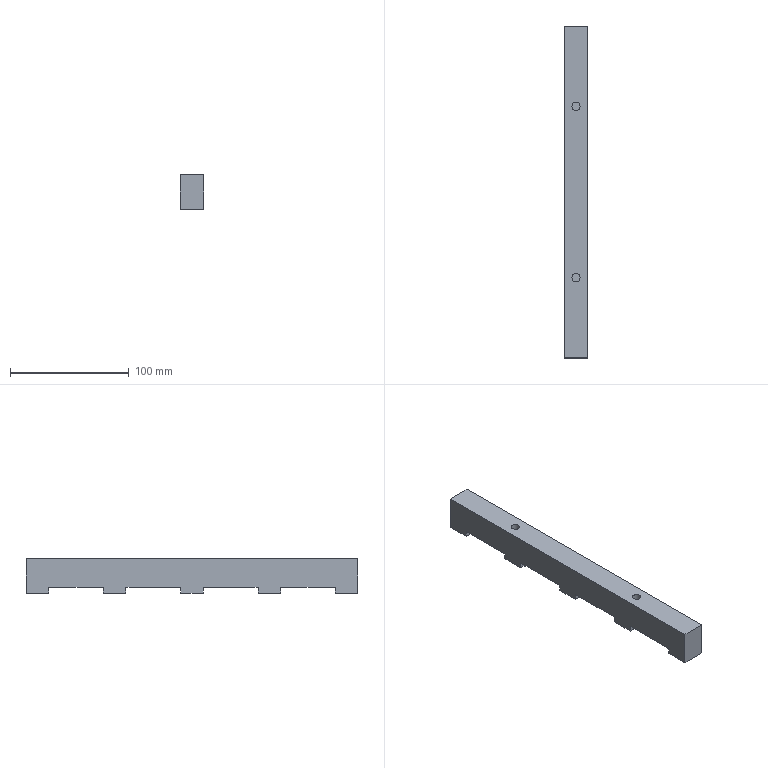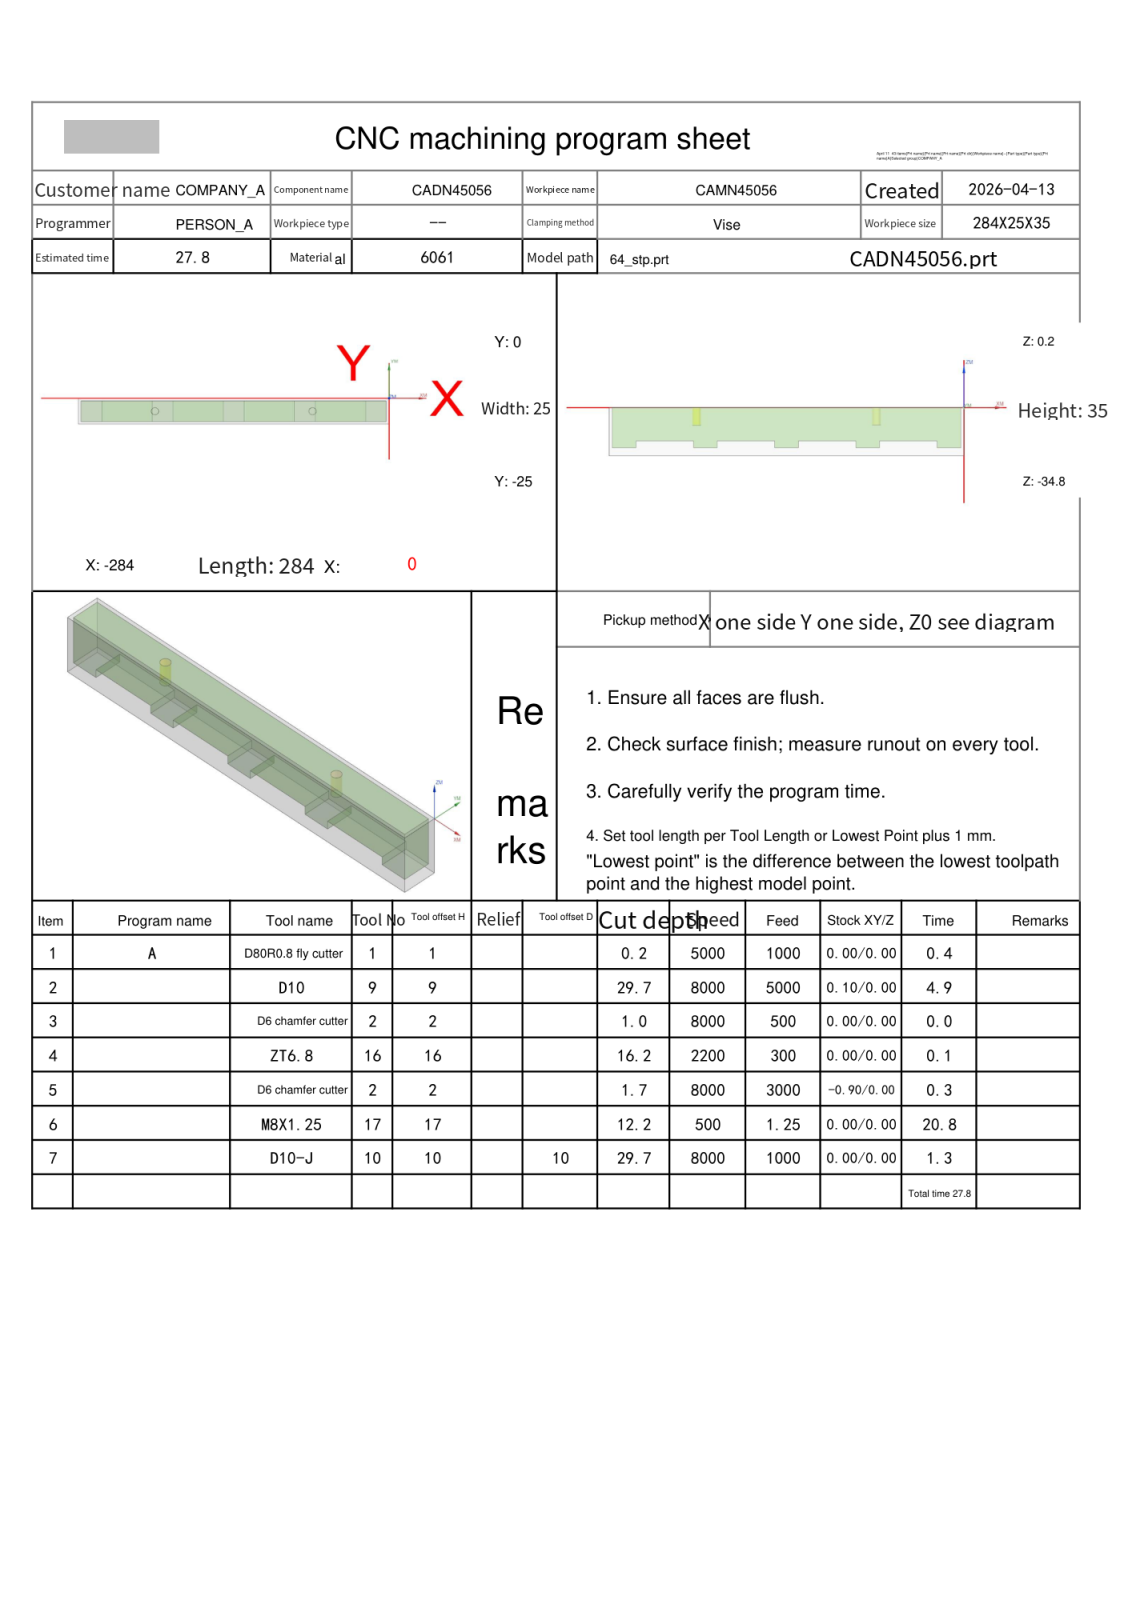NC program | NX | posted by the shop | part box 20 x 279 x 29 mm
Whole program:
%
O0001
(Machine time: 48.52 MIN)
(===Total Tool:6===)
(T1=D80R0.8 fly cutter D=80.  R=0.8  D-  H01 Z=-0.   )
(T9=D10     D=10.  R=0.   D-  H09 Z=-29.5 )
(T2=D6 chamfer cutter   D=6.   R=0.   D-  H02 Z=-1.5  )
(T16=ZT6.8  D=6.8  DR_a=118 D-  H16 Z=-16.  )
(T17=M8X1.25 D=6.8  DR_a=180 D-  H17 Z=-12.  )
(T10=D10-J  D=10.  R=0.   D10 H10 Z=-29.5 )
G80 G90 G17 G49 G40
G91 G28 Z0
M01
N1 T01 M06
(D80R0.8 fly cutter  D=80. R=0.8 H=01 ce=0.00 di=0.00)
G00 G90 G54 X-326.5 Y-12.5 M03 S5000
G43 H01 Z20.
M08
Z2.
G01 Z0.0 F1000.
X-321.5
X37.5
X42.5
Z2.
G00 Z20.
G91 G28 Z0.0
M05
M09
G91 G28 Z0.0
M01
N2 T09 M06
(D10  D=10. R=0. H=09 ce=0.10 di=0.00)
G00 G90 G54 X-142. Y2.6 M03 S8000
G43 H09 Z20.
M08
Z.5
G01 X-2.5 Z.325 F5000.
G02 X2.6 Y-2.5 Z.315 I0.0 J-5.1
G01 Y-22.5 Z.29
G02 X-2.5 Y-27.6 Z.28 I-5.1 J0.0
G01 X-281.5 Z-.07
G02 X-286.6 Y-22.5 Z-.08 I0.0 J5.1
G01 Y-2.5 Z-.105
G02 X-281.5 Y2.6 Z-.115 I5.1 J0.0
G01 X-2.5 Z-.464
G02 X2.6 Y-2.5 Z-.474 I0.0 J-5.1
G01 Y-22.5 Z-.499
G02 X-2.5 Y-27.6 Z-.509 I-5.1 J0.0
G01 X-281.5 Z-.859
G02 X-286.6 Y-22.5 Z-.869 I0.0 J5.1
G01 Y-2.5 Z-.894
G02 X-281.5 Y2.6 Z-.904 I5.1 J0.0
G01 X-2.5 Z-1.254
G02 X2.6 Y-2.5 Z-1.264 I0.0 J-5.1
G01 Y-22.5 Z-1.289
G02 X-2.5 Y-27.6 Z-1.299 I-5.1 J0.0
G01 X-281.5 Z-1.648
G02 X-286.6 Y-22.5 Z-1.659 I0.0 J5.1
G01 Y-2.5 Z-1.684
G02 X-281.5 Y2.6 Z-1.694 I5.1 J0.0
G01 X-2.5 Z-2.043
G02 X2.6 Y-2.5 Z-2.053 I0.0 J-5.1
G01 Y-22.5 Z-2.078
G02 X-2.5 Y-27.6 Z-2.088 I-5.1 J0.0
G01 X-281.5 Z-2.438
G02 X-286.6 Y-22.5 Z-2.448 I0.0 J5.1
G01 Y-2.5 Z-2.473
G02 X-281.5 Y2.6 Z-2.483 I5.1 J0.0
G01 X-2.5 Z-2.833
G02 X2.6 Y-2.5 Z-2.843 I0.0 J-5.1
G01 Y-22.5 Z-2.868
G02 X-2.5 Y-27.6 Z-2.878 I-5.1 J0.0
G01 X-281.5 Z-3.227
G02 X-286.6 Y-22.5 Z-3.237 I0.0 J5.1
G01 Y-2.5 Z-3.263
G02 X-281.5 Y2.6 Z-3.273 I5.1 J0.0
G01 X-2.5 Z-3.622
G02 X2.6 Y-2.5 Z-3.632 I0.0 J-5.1
G01 Y-22.5 Z-3.657
G02 X-2.5 Y-27.6 Z-3.667 I-5.1 J0.0
G01 X-281.5 Z-4.017
G02 X-286.6 Y-22.5 Z-4.027 I0.0 J5.1
G01 Y-2.5 Z-4.052
G02 X-281.5 Y2.6 Z-4.062 I5.1 J0.0
G01 X-2.5 Z-4.412
G02 X2.6 Y-2.5 Z-4.422 I0.0 J-5.1
G01 Y-22.5 Z-4.447
G02 X-2.5 Y-27.6 Z-4.457 I-5.1 J0.0
G01 X-281.5 Z-4.806
G02 X-286.6 Y-22.5 Z-4.816 I0.0 J5.1
G01 Y-2.5 Z-4.841
G02 X-281.5 Y2.6 Z-4.852 I5.1 J0.0
G01 X-2.5 Z-5.201
G02 X2.6 Y-2.5 Z-5.211 I0.0 J-5.1
G01 Y-22.5 Z-5.236
G02 X-2.5 Y-27.6 Z-5.246 I-5.1 J0.0
G01 X-281.5 Z-5.596
G02 X-286.6 Y-22.5 Z-5.606 I0.0 J5.1
G01 Y-2.5 Z-5.631
G02 X-281.5 Y2.6 Z-5.641 I5.1 J0.0
G01 X-2.5 Z-5.991
G02 X2.6 Y-2.5 Z-6.001 I0.0 J-5.1
G01 Y-22.5 Z-6.026
G02 X-2.5 Y-27.6 Z-6.036 I-5.1 J0.0
G01 X-281.5 Z-6.385
G02 X-286.6 Y-22.5 Z-6.395 I0.0 J5.1
G01 Y-2.5 Z-6.42
G02 X-281.5 Y2.6 Z-6.43 I5.1 J0.0
G01 X-2.5 Z-6.78
G02 X2.6 Y-2.5 Z-6.79 I0.0 J-5.1
G01 Y-22.5 Z-6.815
G02 X-2.5 Y-27.6 Z-6.825 I-5.1 J0.0
G01 X-281.5 Z-7.175
G02 X-286.6 Y-22.5 Z-7.185 I0.0 J5.1
G01 Y-2.5 Z-7.21
G02 X-281.5 Y2.6 Z-7.22 I5.1 J0.0
G01 X-2.5 Z-7.57
G02 X2.6 Y-2.5 Z-7.58 I0.0 J-5.1
G01 Y-22.5 Z-7.605
G02 X-2.5 Y-27.6 Z-7.615 I-5.1 J0.0
G01 X-281.5 Z-7.964
G02 X-286.6 Y-22.5 Z-7.974 I0.0 J5.1
G01 Y-2.5 Z-7.999
G02 X-281.5 Y2.6 Z-8.009 I5.1 J0.0
G01 X-2.5 Z-8.359
G02 X2.6 Y-2.5 Z-8.369 I0.0 J-5.1
G01 Y-22.5 Z-8.394
G02 X-2.5 Y-27.6 Z-8.404 I-5.1 J0.0
G01 X-281.5 Z-8.754
G02 X-286.6 Y-22.5 Z-8.764 I0.0 J5.1
G01 Y-2.5 Z-8.789
G02 X-281.5 Y2.6 Z-8.799 I5.1 J0.0
G01 X-2.5 Z-9.148
G02 X2.6 Y-2.5 Z-9.159 I0.0 J-5.1
G01 Y-22.5 Z-9.184
G02 X-2.5 Y-27.6 Z-9.194 I-5.1 J0.0
G01 X-281.5 Z-9.543
G02 X-286.6 Y-22.5 Z-9.553 I0.0 J5.1
G01 Y-2.5 Z-9.578
G02 X-281.5 Y2.6 Z-9.588 I5.1 J0.0
G01 X-2.5 Z-9.938
G02 X2.6 Y-2.5 Z-9.948 I0.0 J-5.1
G01 Y-22.5 Z-9.973
G02 X-2.5 Y-27.6 Z-9.983 I-5.1 J0.0
G01 X-281.5 Z-10.333
G02 X-286.6 Y-22.5 Z-10.343 I0.0 J5.1
G01 Y-2.5 Z-10.368
G02 X-281.5 Y2.6 Z-10.378 I5.1 J0.0
G01 X-2.5 Z-10.727
G02 X2.6 Y-2.5 Z-10.737 I0.0 J-5.1
G01 Y-22.5 Z-10.763
G02 X-2.5 Y-27.6 Z-10.773 I-5.1 J0.0
G01 X-281.5 Z-11.122
G02 X-286.6 Y-22.5 Z-11.132 I0.0 J5.1
G01 Y-2.5 Z-11.157
G02 X-281.5 Y2.6 Z-11.167 I5.1 J0.0
G01 X-2.5 Z-11.517
G02 X2.6 Y-2.5 Z-11.527 I0.0 J-5.1
G01 Y-22.5 Z-11.552
G02 X-2.5 Y-27.6 Z-11.562 I-5.1 J0.0
G01 X-281.5 Z-11.912
G02 X-286.6 Y-22.5 Z-11.922 I0.0 J5.1
G01 Y-2.5 Z-11.947
G02 X-281.5 Y2.6 Z-11.957 I5.1 J0.0
G01 X-2.5 Z-12.306
G02 X2.6 Y-2.5 Z-12.316 I0.0 J-5.1
G01 Y-22.5 Z-12.341
G02 X-2.5 Y-27.6 Z-12.352 I-5.1 J0.0
G01 X-281.5 Z-12.701
G02 X-286.6 Y-22.5 Z-12.711 I0.0 J5.1
G01 Y-2.5 Z-12.736
G02 X-281.5 Y2.6 Z-12.746 I5.1 J0.0
G01 X-2.5 Z-13.096
G02 X2.6 Y-2.5 Z-13.106 I0.0 J-5.1
G01 Y-22.5 Z-13.131
G02 X-2.5 Y-27.6 Z-13.141 I-5.1 J0.0
G01 X-281.5 Z-13.491
G02 X-286.6 Y-22.5 Z-13.501 I0.0 J5.1
G01 Y-2.5 Z-13.526
G02 X-281.5 Y2.6 Z-13.536 I5.1 J0.0
G01 X-2.5 Z-13.885
G02 X2.6 Y-2.5 Z-13.895 I0.0 J-5.1
G01 Y-22.5 Z-13.92
G02 X-2.5 Y-27.6 Z-13.93 I-5.1 J0.0
G01 X-281.5 Z-14.28
G02 X-286.6 Y-22.5 Z-14.29 I0.0 J5.1
G01 Y-2.5 Z-14.315
G02 X-281.5 Y2.6 Z-14.325 I5.1 J0.0
G01 X-2.5 Z-14.675
G02 X2.6 Y-2.5 Z-14.685 I0.0 J-5.1
G01 Y-22.5 Z-14.71
G02 X-2.5 Y-27.6 Z-14.72 I-5.1 J0.0
G01 X-281.5 Z-15.07
G02 X-286.6 Y-22.5 Z-15.08 I0.0 J5.1
G01 Y-2.5 Z-15.105
G02 X-281.5 Y2.6 Z-15.115 I5.1 J0.0
G01 X-2.5 Z-15.464
G02 X2.6 Y-2.5 Z-15.474 I0.0 J-5.1
G01 Y-22.5 Z-15.499
G02 X-2.5 Y-27.6 Z-15.509 I-5.1 J0.0
G01 X-281.5 Z-15.859
G02 X-286.6 Y-22.5 Z-15.869 I0.0 J5.1
G01 Y-2.5 Z-15.894
G02 X-281.5 Y2.6 Z-15.904 I5.1 J0.0
G01 X-2.5 Z-16.254
G02 X2.6 Y-2.5 Z-16.264 I0.0 J-5.1
G01 Y-22.5 Z-16.289
G02 X-2.5 Y-27.6 Z-16.299 I-5.1 J0.0
G01 X-281.5 Z-16.648
G02 X-286.6 Y-22.5 Z-16.659 I0.0 J5.1
G01 Y-2.5 Z-16.684
G02 X-281.5 Y2.6 Z-16.694 I5.1 J0.0
G01 X-2.5 Z-17.043
G02 X2.6 Y-2.5 Z-17.053 I0.0 J-5.1
G01 Y-22.5 Z-17.078
G02 X-2.5 Y-27.6 Z-17.088 I-5.1 J0.0
G01 X-281.5 Z-17.438
G02 X-286.6 Y-22.5 Z-17.448 I0.0 J5.1
G01 Y-2.5 Z-17.473
G02 X-281.5 Y2.6 Z-17.483 I5.1 J0.0
G01 X-2.5 Z-17.833
G02 X2.6 Y-2.5 Z-17.843 I0.0 J-5.1
G01 Y-22.5 Z-17.868
G02 X-2.5 Y-27.6 Z-17.878 I-5.1 J0.0
G01 X-281.5 Z-18.227
G02 X-286.6 Y-22.5 Z-18.237 I0.0 J5.1
G01 Y-2.5 Z-18.263
G02 X-281.5 Y2.6 Z-18.273 I5.1 J0.0
G01 X-2.5 Z-18.622
G02 X2.6 Y-2.5 Z-18.632 I0.0 J-5.1
G01 Y-22.5 Z-18.657
G02 X-2.5 Y-27.6 Z-18.667 I-5.1 J0.0
G01 X-281.5 Z-19.017
G02 X-286.6 Y-22.5 Z-19.027 I0.0 J5.1
G01 Y-2.5 Z-19.052
G02 X-281.5 Y2.6 Z-19.062 I5.1 J0.0
G01 X-2.5 Z-19.412
G02 X2.6 Y-2.5 Z-19.422 I0.0 J-5.1
G01 Y-22.5 Z-19.447
G02 X-2.5 Y-27.6 Z-19.457 I-5.1 J0.0
G01 X-281.5 Z-19.806
G02 X-286.6 Y-22.5 Z-19.816 I0.0 J5.1
G01 Y-2.5 Z-19.841
G02 X-281.5 Y2.6 Z-19.852 I5.1 J0.0
G01 X-2.5 Z-20.201
G02 X2.6 Y-2.5 Z-20.211 I0.0 J-5.1
G01 Y-22.5 Z-20.236
G02 X-2.5 Y-27.6 Z-20.246 I-5.1 J0.0
G01 X-281.5 Z-20.596
G02 X-286.6 Y-22.5 Z-20.606 I0.0 J5.1
G01 Y-2.5 Z-20.631
G02 X-281.5 Y2.6 Z-20.641 I5.1 J0.0
G01 X-2.5 Z-20.991
G02 X2.6 Y-2.5 Z-21.001 I0.0 J-5.1
G01 Y-22.5 Z-21.026
G02 X-2.5 Y-27.6 Z-21.036 I-5.1 J0.0
G01 X-281.5 Z-21.385
G02 X-286.6 Y-22.5 Z-21.395 I0.0 J5.1
G01 Y-2.5 Z-21.42
G02 X-281.5 Y2.6 Z-21.43 I5.1 J0.0
G01 X-2.5 Z-21.78
G02 X2.6 Y-2.5 Z-21.79 I0.0 J-5.1
G01 Y-22.5 Z-21.815
G02 X-2.5 Y-27.6 Z-21.825 I-5.1 J0.0
G01 X-281.5 Z-22.175
G02 X-286.6 Y-22.5 Z-22.185 I0.0 J5.1
G01 Y-2.5 Z-22.21
G02 X-281.5 Y2.6 Z-22.22 I5.1 J0.0
G01 X-2.5 Z-22.57
G02 X2.6 Y-2.5 Z-22.58 I0.0 J-5.1
G01 Y-22.5 Z-22.605
G02 X-2.5 Y-27.6 Z-22.615 I-5.1 J0.0
G01 X-281.5 Z-22.964
G02 X-286.6 Y-22.5 Z-22.974 I0.0 J5.1
G01 Y-2.5 Z-22.999
G02 X-281.5 Y2.6 Z-23.009 I5.1 J0.0
G01 X-2.5 Z-23.359
G02 X2.6 Y-2.5 Z-23.369 I0.0 J-5.1
G01 Y-22.5 Z-23.394
G02 X-2.5 Y-27.6 Z-23.404 I-5.1 J0.0
G01 X-281.5 Z-23.754
G02 X-286.6 Y-22.5 Z-23.764 I0.0 J5.1
G01 Y-2.5 Z-23.789
G02 X-281.5 Y2.6 Z-23.799 I5.1 J0.0
G01 X-2.5 Z-24.148
G02 X2.6 Y-2.5 Z-24.159 I0.0 J-5.1
G01 Y-22.5 Z-24.184
G02 X-2.5 Y-27.6 Z-24.194 I-5.1 J0.0
G01 X-281.5 Z-24.543
G02 X-286.6 Y-22.5 Z-24.553 I0.0 J5.1
G01 Y-2.5 Z-24.578
G02 X-281.5 Y2.6 Z-24.588 I5.1 J0.0
G01 X-2.5 Z-24.938
G02 X2.6 Y-2.5 Z-24.948 I0.0 J-5.1
G01 Y-22.5 Z-24.973
G02 X-2.5 Y-27.6 Z-24.983 I-5.1 J0.0
G01 X-281.5 Z-25.333
G02 X-286.6 Y-22.5 Z-25.343 I0.0 J5.1
G01 Y-2.5 Z-25.368
G02 X-281.5 Y2.6 Z-25.378 I5.1 J0.0
G01 X-2.5 Z-25.727
G02 X2.6 Y-2.5 Z-25.737 I0.0 J-5.1
G01 Y-22.5 Z-25.763
G02 X-2.5 Y-27.6 Z-25.773 I-5.1 J0.0
G01 X-281.5 Z-26.122
G02 X-286.6 Y-22.5 Z-26.132 I0.0 J5.1
G01 Y-2.5 Z-26.157
G02 X-281.5 Y2.6 Z-26.167 I5.1 J0.0
G01 X-2.5 Z-26.517
G02 X2.6 Y-2.5 Z-26.527 I0.0 J-5.1
G01 Y-22.5 Z-26.552
G02 X-2.5 Y-27.6 Z-26.562 I-5.1 J0.0
G01 X-281.5 Z-26.912
G02 X-286.6 Y-22.5 Z-26.922 I0.0 J5.1
G01 Y-2.5 Z-26.947
G02 X-281.5 Y2.6 Z-26.957 I5.1 J0.0
G01 X-2.5 Z-27.306
G02 X2.6 Y-2.5 Z-27.316 I0.0 J-5.1
G01 Y-22.5 Z-27.341
G02 X-2.5 Y-27.6 Z-27.352 I-5.1 J0.0
G01 X-281.5 Z-27.701
G02 X-286.6 Y-22.5 Z-27.711 I0.0 J5.1
G01 Y-2.5 Z-27.736
G02 X-281.5 Y2.6 Z-27.746 I5.1 J0.0
G01 X-2.5 Z-28.096
G02 X2.6 Y-2.5 Z-28.106 I0.0 J-5.1
G01 Y-22.5 Z-28.131
G02 X-2.5 Y-27.6 Z-28.141 I-5.1 J0.0
G01 X-281.5 Z-28.491
G02 X-286.6 Y-22.5 Z-28.501 I0.0 J5.1
G01 Y-2.5 Z-28.526
G02 X-281.5 Y2.6 Z-28.536 I5.1 J0.0
G01 X-2.5 Z-28.885
G02 X2.6 Y-2.5 Z-28.895 I0.0 J-5.1
G01 Y-22.5 Z-28.92
G02 X-2.5 Y-27.6 Z-28.93 I-5.1 J0.0
G01 X-281.5 Z-29.28
G02 X-286.6 Y-22.5 Z-29.29 I0.0 J5.1
G01 Y-2.5 Z-29.315
G02 X-281.5 Y2.6 Z-29.325 I5.1 J0.0
G01 X-142. Z-29.5
X-2.5
G02 X2.6 Y-2.5 I0.0 J-5.1
G01 Y-22.5
G02 X-2.5 Y-27.6 I-5.1 J0.0
G01 X-281.5
G02 X-286.6 Y-22.5 I0.0 J5.1
G01 Y-2.5
G02 X-281.5 Y2.6 I5.1 J0.0
G01 X-142.
X-141.5
Z-28.5
G00 Z20.
G91 G28 Z0.0
M05
M09
G91 G28 Z0.0
M01
N3 T02 M06
(D6 chamfer cutter  D=6. R=0. H=02 ce=0.00 di=0.00)
G00 G90 G54 X-214. Y-12.5 M03 S8000
G43 H02 Z20.
M08
G98 G81 X-214. Y-12.5 Z-.8 R1. F500.
X-70.
G80
G00 Z20.
G91 G28 Z0.0
M05
M09
G91 G28 Z0.0
M01
N4 T16 M06
(ZT6.8 D=6.8 DR_a=118 H=16)
G00 G90 G54 X-214. Y-12.5 M03 S2200
G43 H16 Z20.
M08
G98 G83 X-214. Y-12.5 Z-16. R1. F300. Q2.
X-70.
G80
G00 Z20.
G91 G28 Z0.0
M05
M09
G91 G28 Z0.0
M01
N5 T02 M06
(D6 chamfer cutter  D=6. R=0. H=02 ce=0.00 di=0.00)
G00 G90 G54 X-141.75 Y-24.628 M03 S8000
G43 H02 Z20.
M08
Z2.099
G01 Z-1.499 F3000.
G03 X-141.67 Y-24.328 I-.52 J.3
X-141.97 Y-23.808 I-.6 J0.0
G01 X-142. Y-23.8
X-281.5
G02 X-282.8 Y-22.5 I0.0 J1.3
G01 Y-2.5
G02 X-281.5 Y-1.2 I1.3 J0.0
G01 X-2.5
G02 X-1.2 Y-2.5 I0.0 J-1.3
G01 Y-22.5
G02 X-2.5 Y-23.8 I-1.3 J0.0
G01 X-142.
X-142.03 Y-23.808
G03 X-142.33 Y-24.328 I.3 J-.52
X-142.25 Y-24.628 I.6 J0.0
G01 Z2.099
G00 Z20.
G00 G90 X-212.5 Y-11.27 M03 S8000
Z20.
Z-.9
G01 Z-1.4 F600.
Y-11.06
G03 X-214. Y-9.56 I-1.5 J0.0
X-216.94 Y-12.5 I0.0 J-2.94
X-214. Y-15.44 I2.94 J0.0
X-211.06 Y-12.5 I0.0 J2.94
X-214. Y-9.56 I-2.94 J0.0
X-215.5 Y-11.06 I0.0 J-1.5
G01 Y-11.27
Z-.9
G00 Z20.
X-68.5
Z-.9
G01 Z-1.4
Y-11.06
G03 X-70. Y-9.56 I-1.5 J0.0
X-72.94 Y-12.5 I0.0 J-2.94
X-70. Y-15.44 I2.94 J0.0
X-67.06 Y-12.5 I0.0 J2.94
X-70. Y-9.56 I-2.94 J0.0
X-71.5 Y-11.06 I0.0 J-1.5
G01 Y-11.27
Z-.9
G00 Z20.
G91 G28 Z0.0
M05
M09
G91 G28 Z0.0
M01
N6 T17 M06
(M8X1.25 D=6.8 DR_a=180 H=17)
G00 G90 G54 X-214. Y-12.5 M03 S500
G43 H17 Z20.
M08
G95
G98 G84 X-214. Y-12.5 Z-12. R1. F1.25 Q4.
X-70.
G80
G94
G00 Z20.
G91 G28 Z0.0
M05
M09
G91 G28 Z0.0
M01
N7 T10 M06
(D10-J  D=10. R=0. H=10 ce=0.00 di=0.00)
G00 G90 G54 X-282.513 Y3.616 M03 S8000
G43 H10 Z20.
M08
Z-14.25
G01 Z-14.75 F1000.
G41 D10
X-282.497 Y3.417
G03 X-281.5 Y2.5 I.997 J.083
G01 X-2.5
G02 X2.5 Y-2.5 I0.0 J-5.
G01 Y-22.5
G02 X-2.5 Y-27.5 I-5. J0.0
G01 X-281.5
G02 X-286.5 Y-22.5 I0.0 J5.
G01 Y-2.5
G02 X-281.5 Y2.5 I5. J0.0
G01 X-281.
G03 X-280. Y3.5 I0.0 J1.
G01 G40 Y3.7
Z-14.25
G00 Z20.
X-282.513 Y3.616
Z-29.
G01 Z-29.5
G41 D10
X-282.497 Y3.417
G03 X-281.5 Y2.5 I.997 J.083
G01 X-2.5
G02 X2.5 Y-2.5 I0.0 J-5.
G01 Y-22.5
G02 X-2.5 Y-27.5 I-5. J0.0
G01 X-281.5
G02 X-286.5 Y-22.5 I0.0 J5.
G01 Y-2.5
G02 X-281.5 Y2.5 I5. J0.0
G01 X-281.
G03 X-280. Y3.5 I0.0 J1.
G01 G40 Y3.7
Z-29.
G00 Z20.
M05
M09
G91 G28 Z0.0
G91 G28 Y0.0
M30
%